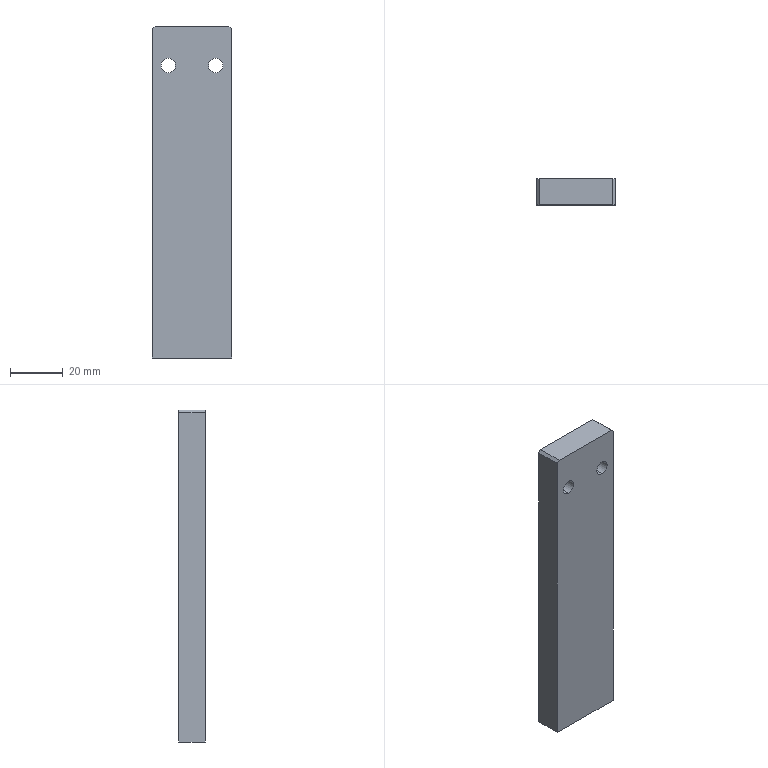Part | SolidWorks | features HoleWzd 2, Chamfer 1, Extrusion 1 | 1 solid | 26 faces | box 30 x 10 x 126 mm | volume 36512 mm3 | cylinder 12 | plane 10 | cone 4 | commonest cylinder face diameters 3.3 x4 5.5 x4 10 x4
STEP:
#1=CARTESIAN_POINT('',(11.65,0.,-52.9));
#2=VERTEX_POINT('',#1);
#3=CARTESIAN_POINT('',(8.35,0.,-52.9));
#4=VERTEX_POINT('',#3);
#5=CARTESIAN_POINT('',(10.,0.,-52.9));
#6=DIRECTION('',(0.,0.,-1.));
#7=DIRECTION('',(-1.,0.,0.));
#8=AXIS2_PLACEMENT_3D('',#5,#6,#7);
#9=CIRCLE('',#8,1.65);
#10=EDGE_CURVE('',#2,#4,#9,.T.);
#11=ORIENTED_EDGE('',*,*,#10,.F.);
#12=CARTESIAN_POINT('',(11.65,0.,-63.));
#13=VERTEX_POINT('',#12);
#14=CARTESIAN_POINT('',(11.65,0.,-63.));
#15=DIRECTION('',(0.,0.,-1.));
#16=VECTOR('',#15,1000.);
#17=LINE('',#14,#16);
#18=EDGE_CURVE('',#2,#13,#17,.T.);
#19=ORIENTED_EDGE('',*,*,#18,.T.);
#20=CARTESIAN_POINT('',(8.35,0.,-63.));
#21=VERTEX_POINT('',#20);
#22=CARTESIAN_POINT('',(10.,0.,-63.));
#23=DIRECTION('',(0.,0.,-1.));
#24=DIRECTION('',(-1.,0.,0.));
#25=AXIS2_PLACEMENT_3D('',#22,#23,#24);
#26=CIRCLE('',#25,1.65);
#27=EDGE_CURVE('',#13,#21,#26,.T.);
#28=ORIENTED_EDGE('',*,*,#27,.T.);
#29=CARTESIAN_POINT('',(8.35,0.,-63.));
#30=DIRECTION('',(0.,0.,-1.));
#31=VECTOR('',#30,1000.);
#32=LINE('',#29,#31);
#33=EDGE_CURVE('',#4,#21,#32,.T.);
#34=ORIENTED_EDGE('',*,*,#33,.F.);
#35=EDGE_LOOP('',(#11,#19,#28,#34));
#36=FACE_OUTER_BOUND('',#35,.T.);
#37=CARTESIAN_POINT('',(10.,0.,-63.));
#38=DIRECTION('',(0.,0.,-1.));
#39=DIRECTION('',(-1.,0.,0.));
#40=AXIS2_PLACEMENT_3D('',#37,#38,#39);
#41=CYLINDRICAL_SURFACE('',#40,1.65);
#42=ADVANCED_FACE('',(#36),#41,.F.);
#43=CARTESIAN_POINT('',(10.,0.,-51.909));
#44=VERTEX_POINT('',#43);
#45=CARTESIAN_POINT('',(8.35,0.,-52.9));
#46=DIRECTION('',(-0.8572,0.,-0.515));
#47=VECTOR('',#46,1000.);
#48=LINE('',#45,#47);
#49=EDGE_CURVE('',#44,#4,#48,.T.);
#50=ORIENTED_EDGE('',*,*,#49,.F.);
#51=CARTESIAN_POINT('',(11.65,0.,-52.9));
#52=DIRECTION('',(0.8572,0.,-0.515));
#53=VECTOR('',#52,1000.);
#54=LINE('',#51,#53);
#55=EDGE_CURVE('',#44,#2,#54,.T.);
#56=ORIENTED_EDGE('',*,*,#55,.T.);
#57=ORIENTED_EDGE('',*,*,#10,.T.);
#58=EDGE_LOOP('',(#50,#56,#57));
#59=FACE_OUTER_BOUND('',#58,.T.);
#60=CARTESIAN_POINT('',(10.,0.,-52.9));
#61=DIRECTION('',(0.,0.,-1.));
#62=DIRECTION('',(-1.,0.,0.));
#63=AXIS2_PLACEMENT_3D('',#60,#61,#62);
#64=CONICAL_SURFACE('',#63,1.65,1.03);
#65=ADVANCED_FACE('',(#59),#64,.F.);
#66=CARTESIAN_POINT('',(-8.35,0.,-52.9));
#67=VERTEX_POINT('',#66);
#68=CARTESIAN_POINT('',(-11.65,0.,-52.9));
#69=VERTEX_POINT('',#68);
#70=CARTESIAN_POINT('',(-10.,0.,-52.9));
#71=DIRECTION('',(0.,0.,-1.));
#72=DIRECTION('',(-1.,0.,0.));
#73=AXIS2_PLACEMENT_3D('',#70,#71,#72);
#74=CIRCLE('',#73,1.65);
#75=EDGE_CURVE('',#67,#69,#74,.T.);
#76=ORIENTED_EDGE('',*,*,#75,.F.);
#77=CARTESIAN_POINT('',(-8.35,0.,-63.));
#78=VERTEX_POINT('',#77);
#79=CARTESIAN_POINT('',(-8.35,0.,-63.));
#80=DIRECTION('',(0.,0.,-1.));
#81=VECTOR('',#80,1000.);
#82=LINE('',#79,#81);
#83=EDGE_CURVE('',#67,#78,#82,.T.);
#84=ORIENTED_EDGE('',*,*,#83,.T.);
#85=CARTESIAN_POINT('',(-11.65,0.,-63.));
#86=VERTEX_POINT('',#85);
#87=CARTESIAN_POINT('',(-10.,0.,-63.));
#88=DIRECTION('',(0.,0.,-1.));
#89=DIRECTION('',(-1.,0.,0.));
#90=AXIS2_PLACEMENT_3D('',#87,#88,#89);
#91=CIRCLE('',#90,1.65);
#92=EDGE_CURVE('',#78,#86,#91,.T.);
#93=ORIENTED_EDGE('',*,*,#92,.T.);
#94=CARTESIAN_POINT('',(-11.65,0.,-63.));
#95=DIRECTION('',(0.,0.,-1.));
#96=VECTOR('',#95,1000.);
#97=LINE('',#94,#96);
#98=EDGE_CURVE('',#69,#86,#97,.T.);
#99=ORIENTED_EDGE('',*,*,#98,.F.);
#100=EDGE_LOOP('',(#76,#84,#93,#99));
#101=FACE_OUTER_BOUND('',#100,.T.);
#102=CARTESIAN_POINT('',(-10.,0.,-63.));
#103=DIRECTION('',(0.,0.,-1.));
#104=DIRECTION('',(-1.,0.,0.));
#105=AXIS2_PLACEMENT_3D('',#102,#103,#104);
#106=CYLINDRICAL_SURFACE('',#105,1.65);
#107=ADVANCED_FACE('',(#101),#106,.F.);
#108=CARTESIAN_POINT('',(-10.,0.,-51.909));
#109=VERTEX_POINT('',#108);
#110=CARTESIAN_POINT('',(-11.65,0.,-52.9));
#111=DIRECTION('',(-0.8572,0.,-0.515));
#112=VECTOR('',#111,1000.);
#113=LINE('',#110,#112);
#114=EDGE_CURVE('',#109,#69,#113,.T.);
#115=ORIENTED_EDGE('',*,*,#114,.F.);
#116=CARTESIAN_POINT('',(-8.35,0.,-52.9));
#117=DIRECTION('',(0.8572,0.,-0.515));
#118=VECTOR('',#117,1000.);
#119=LINE('',#116,#118);
#120=EDGE_CURVE('',#109,#67,#119,.T.);
#121=ORIENTED_EDGE('',*,*,#120,.T.);
#122=ORIENTED_EDGE('',*,*,#75,.T.);
#123=EDGE_LOOP('',(#115,#121,#122));
#124=FACE_OUTER_BOUND('',#123,.T.);
#125=CARTESIAN_POINT('',(-10.,0.,-52.9));
#126=DIRECTION('',(0.,0.,-1.));
#127=DIRECTION('',(-1.,0.,0.));
#128=AXIS2_PLACEMENT_3D('',#125,#126,#127);
#129=CONICAL_SURFACE('',#128,1.65,1.03);
#130=ADVANCED_FACE('',(#124),#129,.F.);
#131=CARTESIAN_POINT('',(9.,-0.7,43.));
#132=VERTEX_POINT('',#131);
#133=CARTESIAN_POINT('',(9.,-0.7,53.));
#134=VERTEX_POINT('',#133);
#135=CARTESIAN_POINT('',(9.,-0.7,48.));
#136=DIRECTION('',(0.,1.,0.));
#137=DIRECTION('',(0.,0.,1.));
#138=AXIS2_PLACEMENT_3D('',#135,#136,#137);
#139=CIRCLE('',#138,5.);
#140=EDGE_CURVE('',#132,#134,#139,.T.);
#141=ORIENTED_EDGE('',*,*,#140,.F.);
#142=CARTESIAN_POINT('',(9.,5.,43.));
#143=VERTEX_POINT('',#142);
#144=CARTESIAN_POINT('',(9.,5.,43.));
#145=DIRECTION('',(0.,1.,0.));
#146=VECTOR('',#145,1000.);
#147=LINE('',#144,#146);
#148=EDGE_CURVE('',#132,#143,#147,.T.);
#149=ORIENTED_EDGE('',*,*,#148,.T.);
#150=CARTESIAN_POINT('',(9.,5.,53.));
#151=VERTEX_POINT('',#150);
#152=CARTESIAN_POINT('',(9.,5.,48.));
#153=DIRECTION('',(0.,1.,0.));
#154=DIRECTION('',(0.,0.,1.));
#155=AXIS2_PLACEMENT_3D('',#152,#153,#154);
#156=CIRCLE('',#155,5.);
#157=EDGE_CURVE('',#143,#151,#156,.T.);
#158=ORIENTED_EDGE('',*,*,#157,.T.);
#159=CARTESIAN_POINT('',(9.,5.,53.));
#160=DIRECTION('',(0.,1.,0.));
#161=VECTOR('',#160,1000.);
#162=LINE('',#159,#161);
#163=EDGE_CURVE('',#134,#151,#162,.T.);
#164=ORIENTED_EDGE('',*,*,#163,.F.);
#165=EDGE_LOOP('',(#141,#149,#158,#164));
#166=FACE_OUTER_BOUND('',#165,.T.);
#167=CARTESIAN_POINT('',(9.,5.,48.));
#168=DIRECTION('',(0.,1.,0.));
#169=DIRECTION('',(0.,0.,1.));
#170=AXIS2_PLACEMENT_3D('',#167,#168,#169);
#171=CYLINDRICAL_SURFACE('',#170,5.);
#172=ADVANCED_FACE('',(#166),#171,.F.);
#173=CARTESIAN_POINT('',(9.,-5.,45.25));
#174=VERTEX_POINT('',#173);
#175=CARTESIAN_POINT('',(9.,-5.,50.75));
#176=VERTEX_POINT('',#175);
#177=CARTESIAN_POINT('',(9.,-5.,48.));
#178=DIRECTION('',(0.,1.,0.));
#179=DIRECTION('',(0.,0.,1.));
#180=AXIS2_PLACEMENT_3D('',#177,#178,#179);
#181=CIRCLE('',#180,2.75);
#182=EDGE_CURVE('',#174,#176,#181,.T.);
#183=ORIENTED_EDGE('',*,*,#182,.F.);
#184=CARTESIAN_POINT('',(9.,-0.7,45.25));
#185=VERTEX_POINT('',#184);
#186=CARTESIAN_POINT('',(9.,5.,45.25));
#187=DIRECTION('',(0.,1.,0.));
#188=VECTOR('',#187,1000.);
#189=LINE('',#186,#188);
#190=EDGE_CURVE('',#174,#185,#189,.T.);
#191=ORIENTED_EDGE('',*,*,#190,.T.);
#192=CARTESIAN_POINT('',(9.,-0.7,50.75));
#193=VERTEX_POINT('',#192);
#194=CARTESIAN_POINT('',(9.,-0.7,48.));
#195=DIRECTION('',(0.,1.,0.));
#196=DIRECTION('',(0.,0.,1.));
#197=AXIS2_PLACEMENT_3D('',#194,#195,#196);
#198=CIRCLE('',#197,2.75);
#199=EDGE_CURVE('',#185,#193,#198,.T.);
#200=ORIENTED_EDGE('',*,*,#199,.T.);
#201=CARTESIAN_POINT('',(9.,5.,50.75));
#202=DIRECTION('',(0.,1.,0.));
#203=VECTOR('',#202,1000.);
#204=LINE('',#201,#203);
#205=EDGE_CURVE('',#176,#193,#204,.T.);
#206=ORIENTED_EDGE('',*,*,#205,.F.);
#207=EDGE_LOOP('',(#183,#191,#200,#206));
#208=FACE_OUTER_BOUND('',#207,.T.);
#209=CARTESIAN_POINT('',(9.,5.,48.));
#210=DIRECTION('',(0.,1.,0.));
#211=DIRECTION('',(0.,0.,1.));
#212=AXIS2_PLACEMENT_3D('',#209,#210,#211);
#213=CYLINDRICAL_SURFACE('',#212,2.75);
#214=ADVANCED_FACE('',(#208),#213,.F.);
#215=CARTESIAN_POINT('',(-9.,-0.7,43.));
#216=VERTEX_POINT('',#215);
#217=CARTESIAN_POINT('',(-9.,-0.7,53.));
#218=VERTEX_POINT('',#217);
#219=CARTESIAN_POINT('',(-9.,-0.7,48.));
#220=DIRECTION('',(0.,1.,0.));
#221=DIRECTION('',(0.,0.,1.));
#222=AXIS2_PLACEMENT_3D('',#219,#220,#221);
#223=CIRCLE('',#222,5.);
#224=EDGE_CURVE('',#216,#218,#223,.T.);
#225=ORIENTED_EDGE('',*,*,#224,.F.);
#226=CARTESIAN_POINT('',(-9.,5.,43.));
#227=VERTEX_POINT('',#226);
#228=CARTESIAN_POINT('',(-9.,5.,43.));
#229=DIRECTION('',(0.,1.,0.));
#230=VECTOR('',#229,1000.);
#231=LINE('',#228,#230);
#232=EDGE_CURVE('',#216,#227,#231,.T.);
#233=ORIENTED_EDGE('',*,*,#232,.T.);
#234=CARTESIAN_POINT('',(-9.,5.,53.));
#235=VERTEX_POINT('',#234);
#236=CARTESIAN_POINT('',(-9.,5.,48.));
#237=DIRECTION('',(0.,1.,0.));
#238=DIRECTION('',(0.,0.,1.));
#239=AXIS2_PLACEMENT_3D('',#236,#237,#238);
#240=CIRCLE('',#239,5.);
#241=EDGE_CURVE('',#227,#235,#240,.T.);
#242=ORIENTED_EDGE('',*,*,#241,.T.);
#243=CARTESIAN_POINT('',(-9.,5.,53.));
#244=DIRECTION('',(0.,1.,0.));
#245=VECTOR('',#244,1000.);
#246=LINE('',#243,#245);
#247=EDGE_CURVE('',#218,#235,#246,.T.);
#248=ORIENTED_EDGE('',*,*,#247,.F.);
#249=EDGE_LOOP('',(#225,#233,#242,#248));
#250=FACE_OUTER_BOUND('',#249,.T.);
#251=CARTESIAN_POINT('',(-9.,5.,48.));
#252=DIRECTION('',(0.,1.,0.));
#253=DIRECTION('',(0.,0.,1.));
#254=AXIS2_PLACEMENT_3D('',#251,#252,#253);
#255=CYLINDRICAL_SURFACE('',#254,5.);
#256=ADVANCED_FACE('',(#250),#255,.F.);
#257=CARTESIAN_POINT('',(-9.,-5.,45.25));
#258=VERTEX_POINT('',#257);
#259=CARTESIAN_POINT('',(-9.,-5.,50.75));
#260=VERTEX_POINT('',#259);
#261=CARTESIAN_POINT('',(-9.,-5.,48.));
#262=DIRECTION('',(0.,1.,0.));
#263=DIRECTION('',(0.,0.,1.));
#264=AXIS2_PLACEMENT_3D('',#261,#262,#263);
#265=CIRCLE('',#264,2.75);
#266=EDGE_CURVE('',#258,#260,#265,.T.);
#267=ORIENTED_EDGE('',*,*,#266,.F.);
#268=CARTESIAN_POINT('',(-9.,-0.7,45.25));
#269=VERTEX_POINT('',#268);
#270=CARTESIAN_POINT('',(-9.,5.,45.25));
#271=DIRECTION('',(0.,1.,0.));
#272=VECTOR('',#271,1000.);
#273=LINE('',#270,#272);
#274=EDGE_CURVE('',#258,#269,#273,.T.);
#275=ORIENTED_EDGE('',*,*,#274,.T.);
#276=CARTESIAN_POINT('',(-9.,-0.7,50.75));
#277=VERTEX_POINT('',#276);
#278=CARTESIAN_POINT('',(-9.,-0.7,48.));
#279=DIRECTION('',(0.,1.,0.));
#280=DIRECTION('',(0.,0.,1.));
#281=AXIS2_PLACEMENT_3D('',#278,#279,#280);
#282=CIRCLE('',#281,2.75);
#283=EDGE_CURVE('',#269,#277,#282,.T.);
#284=ORIENTED_EDGE('',*,*,#283,.T.);
#285=CARTESIAN_POINT('',(-9.,5.,50.75));
#286=DIRECTION('',(0.,1.,0.));
#287=VECTOR('',#286,1000.);
#288=LINE('',#285,#287);
#289=EDGE_CURVE('',#260,#277,#288,.T.);
#290=ORIENTED_EDGE('',*,*,#289,.F.);
#291=EDGE_LOOP('',(#267,#275,#284,#290));
#292=FACE_OUTER_BOUND('',#291,.T.);
#293=CARTESIAN_POINT('',(-9.,5.,48.));
#294=DIRECTION('',(0.,1.,0.));
#295=DIRECTION('',(0.,0.,1.));
#296=AXIS2_PLACEMENT_3D('',#293,#294,#295);
#297=CYLINDRICAL_SURFACE('',#296,2.75);
#298=ADVANCED_FACE('',(#292),#297,.F.);
#299=CARTESIAN_POINT('',(15.,5.,62.));
#300=VERTEX_POINT('',#299);
#301=CARTESIAN_POINT('',(15.,5.,-63.));
#302=VERTEX_POINT('',#301);
#303=CARTESIAN_POINT('',(15.,5.,63.));
#304=DIRECTION('',(0.,0.,-1.));
#305=VECTOR('',#304,1000.);
#306=LINE('',#303,#305);
#307=EDGE_CURVE('',#300,#302,#306,.T.);
#308=ORIENTED_EDGE('',*,*,#307,.F.);
#309=CARTESIAN_POINT('',(15.,-5.,62.));
#310=VERTEX_POINT('',#309);
#311=CARTESIAN_POINT('',(15.,5.,62.));
#312=DIRECTION('',(0.,-1.,0.));
#313=VECTOR('',#312,1000.);
#314=LINE('',#311,#313);
#315=EDGE_CURVE('',#300,#310,#314,.T.);
#316=ORIENTED_EDGE('',*,*,#315,.T.);
#317=CARTESIAN_POINT('',(15.,-5.,-63.));
#318=VERTEX_POINT('',#317);
#319=CARTESIAN_POINT('',(15.,-5.,63.));
#320=DIRECTION('',(0.,0.,-1.));
#321=VECTOR('',#320,1000.);
#322=LINE('',#319,#321);
#323=EDGE_CURVE('',#310,#318,#322,.T.);
#324=ORIENTED_EDGE('',*,*,#323,.T.);
#325=CARTESIAN_POINT('',(15.,5.,-63.));
#326=DIRECTION('',(0.,-1.,0.));
#327=VECTOR('',#326,1000.);
#328=LINE('',#325,#327);
#329=EDGE_CURVE('',#302,#318,#328,.T.);
#330=ORIENTED_EDGE('',*,*,#329,.F.);
#331=EDGE_LOOP('',(#308,#316,#324,#330));
#332=FACE_OUTER_BOUND('',#331,.T.);
#333=CARTESIAN_POINT('',(15.,5.,63.));
#334=DIRECTION('',(-1.,0.,0.));
#335=DIRECTION('',(0.,0.,1.));
#336=AXIS2_PLACEMENT_3D('',#333,#334,#335);
#337=PLANE('',#336);
#338=ADVANCED_FACE('',(#332),#337,.F.);
#339=CARTESIAN_POINT('',(10.,0.,-63.));
#340=DIRECTION('',(0.,0.,-1.));
#341=DIRECTION('',(-1.,0.,0.));
#342=AXIS2_PLACEMENT_3D('',#339,#340,#341);
#343=CIRCLE('',#342,1.65);
#344=EDGE_CURVE('',#21,#13,#343,.T.);
#345=ORIENTED_EDGE('',*,*,#344,.F.);
#346=ORIENTED_EDGE('',*,*,#27,.F.);
#347=EDGE_LOOP('',(#345,#346));
#348=FACE_BOUND('',#347,.T.);
#349=CARTESIAN_POINT('',(-10.,0.,-63.));
#350=DIRECTION('',(0.,0.,-1.));
#351=DIRECTION('',(-1.,0.,0.));
#352=AXIS2_PLACEMENT_3D('',#349,#350,#351);
#353=CIRCLE('',#352,1.65);
#354=EDGE_CURVE('',#86,#78,#353,.T.);
#355=ORIENTED_EDGE('',*,*,#354,.F.);
#356=ORIENTED_EDGE('',*,*,#92,.F.);
#357=EDGE_LOOP('',(#355,#356));
#358=FACE_BOUND('',#357,.T.);
#359=CARTESIAN_POINT('',(-15.,-5.,-63.));
#360=VERTEX_POINT('',#359);
#361=CARTESIAN_POINT('',(-15.,-5.,-63.));
#362=DIRECTION('',(-1.,0.,0.));
#363=VECTOR('',#362,1000.);
#364=LINE('',#361,#363);
#365=EDGE_CURVE('',#318,#360,#364,.T.);
#366=ORIENTED_EDGE('',*,*,#365,.T.);
#367=CARTESIAN_POINT('',(-15.,5.,-63.));
#368=VERTEX_POINT('',#367);
#369=CARTESIAN_POINT('',(-15.,5.,-63.));
#370=DIRECTION('',(0.,-1.,0.));
#371=VECTOR('',#370,1000.);
#372=LINE('',#369,#371);
#373=EDGE_CURVE('',#368,#360,#372,.T.);
#374=ORIENTED_EDGE('',*,*,#373,.F.);
#375=CARTESIAN_POINT('',(-15.,5.,-63.));
#376=DIRECTION('',(-1.,0.,0.));
#377=VECTOR('',#376,1000.);
#378=LINE('',#375,#377);
#379=EDGE_CURVE('',#302,#368,#378,.T.);
#380=ORIENTED_EDGE('',*,*,#379,.F.);
#381=ORIENTED_EDGE('',*,*,#329,.T.);
#382=EDGE_LOOP('',(#366,#374,#380,#381));
#383=FACE_OUTER_BOUND('',#382,.T.);
#384=CARTESIAN_POINT('',(-15.,5.,-63.));
#385=DIRECTION('',(0.,0.,1.));
#386=DIRECTION('',(1.,0.,0.));
#387=AXIS2_PLACEMENT_3D('',#384,#385,#386);
#388=PLANE('',#387);
#389=ADVANCED_FACE('',(#348,#358,#383),#388,.F.);
#390=CARTESIAN_POINT('',(-15.,-5.,62.));
#391=VERTEX_POINT('',#390);
#392=CARTESIAN_POINT('',(-15.,-5.,63.));
#393=DIRECTION('',(0.,0.,1.));
#394=VECTOR('',#393,1000.);
#395=LINE('',#392,#394);
#396=EDGE_CURVE('',#360,#391,#395,.T.);
#397=ORIENTED_EDGE('',*,*,#396,.T.);
#398=CARTESIAN_POINT('',(-15.,5.,62.));
#399=VERTEX_POINT('',#398);
#400=CARTESIAN_POINT('',(-15.,5.,62.));
#401=DIRECTION('',(0.,1.,0.));
#402=VECTOR('',#401,1000.);
#403=LINE('',#400,#402);
#404=EDGE_CURVE('',#391,#399,#403,.T.);
#405=ORIENTED_EDGE('',*,*,#404,.T.);
#406=CARTESIAN_POINT('',(-15.,5.,63.));
#407=DIRECTION('',(0.,0.,1.));
#408=VECTOR('',#407,1000.);
#409=LINE('',#406,#408);
#410=EDGE_CURVE('',#368,#399,#409,.T.);
#411=ORIENTED_EDGE('',*,*,#410,.F.);
#412=ORIENTED_EDGE('',*,*,#373,.T.);
#413=EDGE_LOOP('',(#397,#405,#411,#412));
#414=FACE_OUTER_BOUND('',#413,.T.);
#415=CARTESIAN_POINT('',(-15.,5.,63.));
#416=DIRECTION('',(1.,0.,0.));
#417=DIRECTION('',(0.,0.,-1.));
#418=AXIS2_PLACEMENT_3D('',#415,#416,#417);
#419=PLANE('',#418);
#420=ADVANCED_FACE('',(#414),#419,.F.);
#421=CARTESIAN_POINT('',(-14.,-5.,63.));
#422=VERTEX_POINT('',#421);
#423=CARTESIAN_POINT('',(14.,-5.,63.));
#424=VERTEX_POINT('',#423);
#425=CARTESIAN_POINT('',(-15.,-5.,63.));
#426=DIRECTION('',(1.,0.,0.));
#427=VECTOR('',#426,1000.);
#428=LINE('',#425,#427);
#429=EDGE_CURVE('',#422,#424,#428,.T.);
#430=ORIENTED_EDGE('',*,*,#429,.T.);
#431=CARTESIAN_POINT('',(14.,5.,63.));
#432=VERTEX_POINT('',#431);
#433=CARTESIAN_POINT('',(14.,5.,63.));
#434=DIRECTION('',(0.,1.,0.));
#435=VECTOR('',#434,1000.);
#436=LINE('',#433,#435);
#437=EDGE_CURVE('',#424,#432,#436,.T.);
#438=ORIENTED_EDGE('',*,*,#437,.T.);
#439=CARTESIAN_POINT('',(-14.,5.,63.));
#440=VERTEX_POINT('',#439);
#441=CARTESIAN_POINT('',(-15.,5.,63.));
#442=DIRECTION('',(1.,0.,0.));
#443=VECTOR('',#442,1000.);
#444=LINE('',#441,#443);
#445=EDGE_CURVE('',#440,#432,#444,.T.);
#446=ORIENTED_EDGE('',*,*,#445,.F.);
#447=CARTESIAN_POINT('',(-14.,5.,63.));
#448=DIRECTION('',(0.,-1.,0.));
#449=VECTOR('',#448,1000.);
#450=LINE('',#447,#449);
#451=EDGE_CURVE('',#440,#422,#450,.T.);
#452=ORIENTED_EDGE('',*,*,#451,.T.);
#453=EDGE_LOOP('',(#430,#438,#446,#452));
#454=FACE_OUTER_BOUND('',#453,.T.);
#455=CARTESIAN_POINT('',(-15.,5.,63.));
#456=DIRECTION('',(0.,0.,-1.));
#457=DIRECTION('',(-1.,0.,0.));
#458=AXIS2_PLACEMENT_3D('',#455,#456,#457);
#459=PLANE('',#458);
#460=ADVANCED_FACE('',(#454),#459,.F.);
#461=CARTESIAN_POINT('',(9.,5.,48.));
#462=DIRECTION('',(0.,1.,0.));
#463=DIRECTION('',(0.,0.,1.));
#464=AXIS2_PLACEMENT_3D('',#461,#462,#463);
#465=CIRCLE('',#464,5.);
#466=EDGE_CURVE('',#151,#143,#465,.T.);
#467=ORIENTED_EDGE('',*,*,#466,.F.);
#468=ORIENTED_EDGE('',*,*,#157,.F.);
#469=EDGE_LOOP('',(#467,#468));
#470=FACE_BOUND('',#469,.T.);
#471=CARTESIAN_POINT('',(-9.,5.,48.));
#472=DIRECTION('',(0.,1.,0.));
#473=DIRECTION('',(0.,0.,1.));
#474=AXIS2_PLACEMENT_3D('',#471,#472,#473);
#475=CIRCLE('',#474,5.);
#476=EDGE_CURVE('',#235,#227,#475,.T.);
#477=ORIENTED_EDGE('',*,*,#476,.F.);
#478=ORIENTED_EDGE('',*,*,#241,.F.);
#479=EDGE_LOOP('',(#477,#478));
#480=FACE_BOUND('',#479,.T.);
#481=ORIENTED_EDGE('',*,*,#445,.T.);
#482=CARTESIAN_POINT('',(15.,5.,62.));
#483=DIRECTION('',(0.7071,0.,-0.7071));
#484=VECTOR('',#483,1000.);
#485=LINE('',#482,#484);
#486=EDGE_CURVE('',#432,#300,#485,.T.);
#487=ORIENTED_EDGE('',*,*,#486,.T.);
#488=ORIENTED_EDGE('',*,*,#307,.T.);
#489=ORIENTED_EDGE('',*,*,#379,.T.);
#490=ORIENTED_EDGE('',*,*,#410,.T.);
#491=CARTESIAN_POINT('',(-14.,5.,63.));
#492=DIRECTION('',(0.7071,0.,0.7071));
#493=VECTOR('',#492,1000.);
#494=LINE('',#491,#493);
#495=EDGE_CURVE('',#399,#440,#494,.T.);
#496=ORIENTED_EDGE('',*,*,#495,.T.);
#497=EDGE_LOOP('',(#481,#487,#488,#489,#490,#496));
#498=FACE_OUTER_BOUND('',#497,.T.);
#499=CARTESIAN_POINT('',(0.,5.,0.));
#500=DIRECTION('',(0.,-1.,0.));
#501=DIRECTION('',(0.,0.,-1.));
#502=AXIS2_PLACEMENT_3D('',#499,#500,#501);
#503=PLANE('',#502);
#504=ADVANCED_FACE('',(#470,#480,#498),#503,.F.);
#505=CARTESIAN_POINT('',(9.,-5.,48.));
#506=DIRECTION('',(0.,1.,0.));
#507=DIRECTION('',(0.,0.,1.));
#508=AXIS2_PLACEMENT_3D('',#505,#506,#507);
#509=CIRCLE('',#508,2.75);
#510=EDGE_CURVE('',#176,#174,#509,.T.);
#511=ORIENTED_EDGE('',*,*,#510,.T.);
#512=ORIENTED_EDGE('',*,*,#182,.T.);
#513=EDGE_LOOP('',(#511,#512));
#514=FACE_BOUND('',#513,.T.);
#515=CARTESIAN_POINT('',(-9.,-5.,48.));
#516=DIRECTION('',(0.,1.,0.));
#517=DIRECTION('',(0.,0.,1.));
#518=AXIS2_PLACEMENT_3D('',#515,#516,#517);
#519=CIRCLE('',#518,2.75);
#520=EDGE_CURVE('',#260,#258,#519,.T.);
#521=ORIENTED_EDGE('',*,*,#520,.T.);
#522=ORIENTED_EDGE('',*,*,#266,.T.);
#523=EDGE_LOOP('',(#521,#522));
#524=FACE_BOUND('',#523,.T.);
#525=ORIENTED_EDGE('',*,*,#323,.F.);
#526=CARTESIAN_POINT('',(38.5,-5.,38.5));
#527=DIRECTION('',(-0.7071,0.,0.7071));
#528=VECTOR('',#527,1000.);
#529=LINE('',#526,#528);
#530=EDGE_CURVE('',#310,#424,#529,.T.);
#531=ORIENTED_EDGE('',*,*,#530,.T.);
#532=ORIENTED_EDGE('',*,*,#429,.F.);
#533=CARTESIAN_POINT('',(-38.5,-5.,38.5));
#534=DIRECTION('',(-0.7071,0.,-0.7071));
#535=VECTOR('',#534,1000.);
#536=LINE('',#533,#535);
#537=EDGE_CURVE('',#422,#391,#536,.T.);
#538=ORIENTED_EDGE('',*,*,#537,.T.);
#539=ORIENTED_EDGE('',*,*,#396,.F.);
#540=ORIENTED_EDGE('',*,*,#365,.F.);
#541=EDGE_LOOP('',(#525,#531,#532,#538,#539,#540));
#542=FACE_OUTER_BOUND('',#541,.T.);
#543=CARTESIAN_POINT('',(0.,-5.,0.));
#544=DIRECTION('',(0.,-1.,0.));
#545=DIRECTION('',(0.,0.,-1.));
#546=AXIS2_PLACEMENT_3D('',#543,#544,#545);
#547=PLANE('',#546);
#548=ADVANCED_FACE('',(#514,#524,#542),#547,.T.);
#549=ORIENTED_EDGE('',*,*,#274,.F.);
#550=ORIENTED_EDGE('',*,*,#520,.F.);
#551=ORIENTED_EDGE('',*,*,#289,.T.);
#552=CARTESIAN_POINT('',(-9.,-0.7,48.));
#553=DIRECTION('',(0.,1.,0.));
#554=DIRECTION('',(0.,0.,1.));
#555=AXIS2_PLACEMENT_3D('',#552,#553,#554);
#556=CIRCLE('',#555,2.75);
#557=EDGE_CURVE('',#277,#269,#556,.T.);
#558=ORIENTED_EDGE('',*,*,#557,.T.);
#559=EDGE_LOOP('',(#549,#550,#551,#558));
#560=FACE_OUTER_BOUND('',#559,.T.);
#561=CARTESIAN_POINT('',(-9.,5.,48.));
#562=DIRECTION('',(0.,1.,0.));
#563=DIRECTION('',(0.,0.,1.));
#564=AXIS2_PLACEMENT_3D('',#561,#562,#563);
#565=CYLINDRICAL_SURFACE('',#564,2.75);
#566=ADVANCED_FACE('',(#560),#565,.F.);
#567=ORIENTED_EDGE('',*,*,#557,.F.);
#568=ORIENTED_EDGE('',*,*,#283,.F.);
#569=EDGE_LOOP('',(#567,#568));
#570=FACE_BOUND('',#569,.T.);
#571=CARTESIAN_POINT('',(-9.,-0.7,48.));
#572=DIRECTION('',(0.,1.,0.));
#573=DIRECTION('',(0.,0.,1.));
#574=AXIS2_PLACEMENT_3D('',#571,#572,#573);
#575=CIRCLE('',#574,5.);
#576=EDGE_CURVE('',#218,#216,#575,.T.);
#577=ORIENTED_EDGE('',*,*,#576,.T.);
#578=ORIENTED_EDGE('',*,*,#224,.T.);
#579=EDGE_LOOP('',(#577,#578));
#580=FACE_OUTER_BOUND('',#579,.T.);
#581=CARTESIAN_POINT('',(-6.25,-0.7,48.));
#582=DIRECTION('',(0.,-1.,0.));
#583=DIRECTION('',(0.,0.,-1.));
#584=AXIS2_PLACEMENT_3D('',#581,#582,#583);
#585=PLANE('',#584);
#586=ADVANCED_FACE('',(#570,#580),#585,.F.);
#587=ORIENTED_EDGE('',*,*,#232,.F.);
#588=ORIENTED_EDGE('',*,*,#576,.F.);
#589=ORIENTED_EDGE('',*,*,#247,.T.);
#590=ORIENTED_EDGE('',*,*,#476,.T.);
#591=EDGE_LOOP('',(#587,#588,#589,#590));
#592=FACE_OUTER_BOUND('',#591,.T.);
#593=CARTESIAN_POINT('',(-9.,5.,48.));
#594=DIRECTION('',(0.,1.,0.));
#595=DIRECTION('',(0.,0.,1.));
#596=AXIS2_PLACEMENT_3D('',#593,#594,#595);
#597=CYLINDRICAL_SURFACE('',#596,5.);
#598=ADVANCED_FACE('',(#592),#597,.F.);
#599=ORIENTED_EDGE('',*,*,#190,.F.);
#600=ORIENTED_EDGE('',*,*,#510,.F.);
#601=ORIENTED_EDGE('',*,*,#205,.T.);
#602=CARTESIAN_POINT('',(9.,-0.7,48.));
#603=DIRECTION('',(0.,1.,0.));
#604=DIRECTION('',(0.,0.,1.));
#605=AXIS2_PLACEMENT_3D('',#602,#603,#604);
#606=CIRCLE('',#605,2.75);
#607=EDGE_CURVE('',#193,#185,#606,.T.);
#608=ORIENTED_EDGE('',*,*,#607,.T.);
#609=EDGE_LOOP('',(#599,#600,#601,#608));
#610=FACE_OUTER_BOUND('',#609,.T.);
#611=CARTESIAN_POINT('',(9.,5.,48.));
#612=DIRECTION('',(0.,1.,0.));
#613=DIRECTION('',(0.,0.,1.));
#614=AXIS2_PLACEMENT_3D('',#611,#612,#613);
#615=CYLINDRICAL_SURFACE('',#614,2.75);
#616=ADVANCED_FACE('',(#610),#615,.F.);
#617=ORIENTED_EDGE('',*,*,#607,.F.);
#618=ORIENTED_EDGE('',*,*,#199,.F.);
#619=EDGE_LOOP('',(#617,#618));
#620=FACE_BOUND('',#619,.T.);
#621=CARTESIAN_POINT('',(9.,-0.7,48.));
#622=DIRECTION('',(0.,1.,0.));
#623=DIRECTION('',(0.,0.,1.));
#624=AXIS2_PLACEMENT_3D('',#621,#622,#623);
#625=CIRCLE('',#624,5.);
#626=EDGE_CURVE('',#134,#132,#625,.T.);
#627=ORIENTED_EDGE('',*,*,#626,.T.);
#628=ORIENTED_EDGE('',*,*,#140,.T.);
#629=EDGE_LOOP('',(#627,#628));
#630=FACE_OUTER_BOUND('',#629,.T.);
#631=CARTESIAN_POINT('',(11.75,-0.7,48.));
#632=DIRECTION('',(0.,-1.,0.));
#633=DIRECTION('',(0.,0.,-1.));
#634=AXIS2_PLACEMENT_3D('',#631,#632,#633);
#635=PLANE('',#634);
#636=ADVANCED_FACE('',(#620,#630),#635,.F.);
#637=ORIENTED_EDGE('',*,*,#148,.F.);
#638=ORIENTED_EDGE('',*,*,#626,.F.);
#639=ORIENTED_EDGE('',*,*,#163,.T.);
#640=ORIENTED_EDGE('',*,*,#466,.T.);
#641=EDGE_LOOP('',(#637,#638,#639,#640));
#642=FACE_OUTER_BOUND('',#641,.T.);
#643=CARTESIAN_POINT('',(9.,5.,48.));
#644=DIRECTION('',(0.,1.,0.));
#645=DIRECTION('',(0.,0.,1.));
#646=AXIS2_PLACEMENT_3D('',#643,#644,#645);
#647=CYLINDRICAL_SURFACE('',#646,5.);
#648=ADVANCED_FACE('',(#642),#647,.F.);
#649=ORIENTED_EDGE('',*,*,#486,.F.);
#650=ORIENTED_EDGE('',*,*,#437,.F.);
#651=ORIENTED_EDGE('',*,*,#530,.F.);
#652=ORIENTED_EDGE('',*,*,#315,.F.);
#653=EDGE_LOOP('',(#649,#650,#651,#652));
#654=FACE_OUTER_BOUND('',#653,.T.);
#655=CARTESIAN_POINT('',(15.,5.,62.));
#656=DIRECTION('',(-0.7071,0.,-0.7071));
#657=DIRECTION('',(0.,-1.,0.));
#658=AXIS2_PLACEMENT_3D('',#655,#656,#657);
#659=PLANE('',#658);
#660=ADVANCED_FACE('',(#654),#659,.F.);
#661=ORIENTED_EDGE('',*,*,#495,.F.);
#662=ORIENTED_EDGE('',*,*,#404,.F.);
#663=ORIENTED_EDGE('',*,*,#537,.F.);
#664=ORIENTED_EDGE('',*,*,#451,.F.);
#665=EDGE_LOOP('',(#661,#662,#663,#664));
#666=FACE_OUTER_BOUND('',#665,.T.);
#667=CARTESIAN_POINT('',(-14.,5.,63.));
#668=DIRECTION('',(0.7071,0.,-0.7071));
#669=DIRECTION('',(0.,-1.,0.));
#670=AXIS2_PLACEMENT_3D('',#667,#668,#669);
#671=PLANE('',#670);
#672=ADVANCED_FACE('',(#666),#671,.F.);
#673=ORIENTED_EDGE('',*,*,#120,.F.);
#674=ORIENTED_EDGE('',*,*,#114,.T.);
#675=CARTESIAN_POINT('',(-10.,0.,-52.9));
#676=DIRECTION('',(0.,0.,-1.));
#677=DIRECTION('',(-1.,0.,0.));
#678=AXIS2_PLACEMENT_3D('',#675,#676,#677);
#679=CIRCLE('',#678,1.65);
#680=EDGE_CURVE('',#69,#67,#679,.T.);
#681=ORIENTED_EDGE('',*,*,#680,.T.);
#682=EDGE_LOOP('',(#673,#674,#681));
#683=FACE_OUTER_BOUND('',#682,.T.);
#684=CARTESIAN_POINT('',(-10.,0.,-52.9));
#685=DIRECTION('',(0.,0.,-1.));
#686=DIRECTION('',(-1.,0.,0.));
#687=AXIS2_PLACEMENT_3D('',#684,#685,#686);
#688=CONICAL_SURFACE('',#687,1.65,1.03);
#689=ADVANCED_FACE('',(#683),#688,.F.);
#690=ORIENTED_EDGE('',*,*,#83,.F.);
#691=ORIENTED_EDGE('',*,*,#680,.F.);
#692=ORIENTED_EDGE('',*,*,#98,.T.);
#693=ORIENTED_EDGE('',*,*,#354,.T.);
#694=EDGE_LOOP('',(#690,#691,#692,#693));
#695=FACE_OUTER_BOUND('',#694,.T.);
#696=CARTESIAN_POINT('',(-10.,0.,-63.));
#697=DIRECTION('',(0.,0.,-1.));
#698=DIRECTION('',(-1.,0.,0.));
#699=AXIS2_PLACEMENT_3D('',#696,#697,#698);
#700=CYLINDRICAL_SURFACE('',#699,1.65);
#701=ADVANCED_FACE('',(#695),#700,.F.);
#702=ORIENTED_EDGE('',*,*,#55,.F.);
#703=ORIENTED_EDGE('',*,*,#49,.T.);
#704=CARTESIAN_POINT('',(10.,0.,-52.9));
#705=DIRECTION('',(0.,0.,-1.));
#706=DIRECTION('',(-1.,0.,0.));
#707=AXIS2_PLACEMENT_3D('',#704,#705,#706);
#708=CIRCLE('',#707,1.65);
#709=EDGE_CURVE('',#4,#2,#708,.T.);
#710=ORIENTED_EDGE('',*,*,#709,.T.);
#711=EDGE_LOOP('',(#702,#703,#710));
#712=FACE_OUTER_BOUND('',#711,.T.);
#713=CARTESIAN_POINT('',(10.,0.,-52.9));
#714=DIRECTION('',(0.,0.,-1.));
#715=DIRECTION('',(-1.,0.,0.));
#716=AXIS2_PLACEMENT_3D('',#713,#714,#715);
#717=CONICAL_SURFACE('',#716,1.65,1.03);
#718=ADVANCED_FACE('',(#712),#717,.F.);
#719=ORIENTED_EDGE('',*,*,#18,.F.);
#720=ORIENTED_EDGE('',*,*,#709,.F.);
#721=ORIENTED_EDGE('',*,*,#33,.T.);
#722=ORIENTED_EDGE('',*,*,#344,.T.);
#723=EDGE_LOOP('',(#719,#720,#721,#722));
#724=FACE_OUTER_BOUND('',#723,.T.);
#725=CARTESIAN_POINT('',(10.,0.,-63.));
#726=DIRECTION('',(0.,0.,-1.));
#727=DIRECTION('',(-1.,0.,0.));
#728=AXIS2_PLACEMENT_3D('',#725,#726,#727);
#729=CYLINDRICAL_SURFACE('',#728,1.65);
#730=ADVANCED_FACE('',(#724),#729,.F.);
#731=CLOSED_SHELL('',(#42,#65,#107,#130,#172,#214,#256,#298,#338,#389,#420,#460,#504,#548,#566,#586,#598,#616,#636,#648,#660,#672,#689,#701,#718,#730));
#732=MANIFOLD_SOLID_BREP('',#731);
#733=CARTESIAN_POINT('',(0.,0.,0.));
#734=DIRECTION('',(0.,0.,1.));
#735=DIRECTION('',(1.,0.,0.));
#736=AXIS2_PLACEMENT_3D('',#733,#734,#735);
#737=(LENGTH_UNIT()NAMED_UNIT(*)SI_UNIT(.MILLI.,.METRE.));
#738=UNCERTAINTY_MEASURE_WITH_UNIT(LENGTH_MEASURE(0.00001),#737,'','');
#739=(NAMED_UNIT(*)PLANE_ANGLE_UNIT()SI_UNIT($,.RADIAN.));
#740=(NAMED_UNIT(*)SI_UNIT($,.STERADIAN.)SOLID_ANGLE_UNIT());
#741=(GEOMETRIC_REPRESENTATION_CONTEXT(3)GLOBAL_UNCERTAINTY_ASSIGNED_CONTEXT((#738))GLOBAL_UNIT_ASSIGNED_CONTEXT((#737,#739,#740))REPRESENTATION_CONTEXT('',''));
#742=ADVANCED_BREP_SHAPE_REPRESENTATION('',(#732,#736),#741);